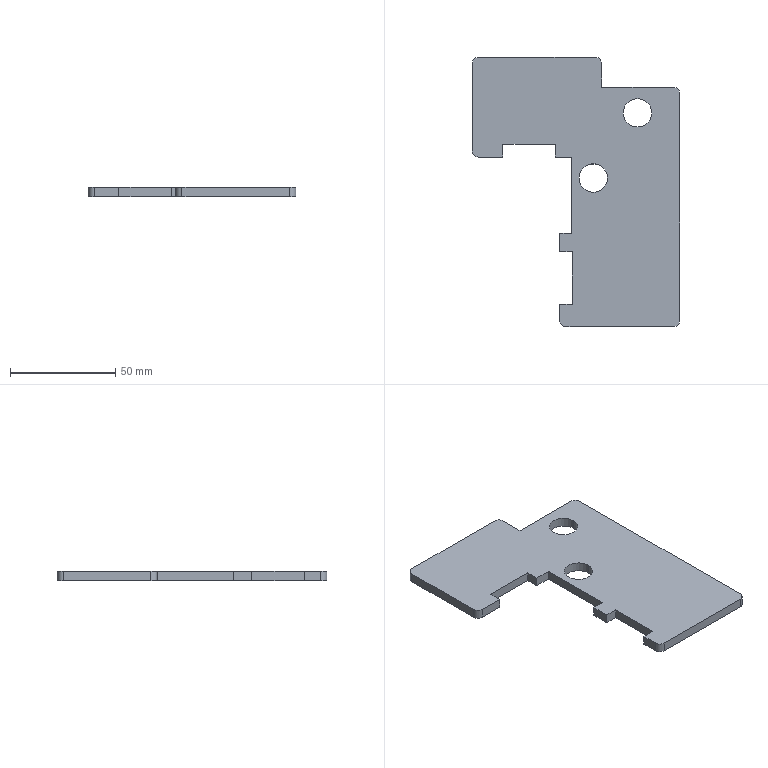Part | SolidWorks | features FlatPattern 1, SMBaseFlange 1, SheetMetal 1 | 1 solid | 30 faces | box 98.706 x 128.023 x 4.5 mm | volume 35781 mm3 | plane 20 | cylinder 10 | commonest cylinder face diameters 6 x6 13.5 x4
STEP:
#1=CARTESIAN_POINT('',(17799.004,-96072.131,-4.5));
#2=VERTEX_POINT('',#1);
#3=CARTESIAN_POINT('',(17812.504,-96072.131,-4.5));
#4=VERTEX_POINT('',#3);
#5=CARTESIAN_POINT('',(17805.754,-96072.131,-4.5));
#6=DIRECTION('',(0.,0.,1.));
#7=DIRECTION('',(1.,0.,0.));
#8=AXIS2_PLACEMENT_3D('',#5,#6,#7);
#9=CIRCLE('',#8,6.75);
#10=EDGE_CURVE('',#2,#4,#9,.T.);
#11=ORIENTED_EDGE('',*,*,#10,.F.);
#12=CARTESIAN_POINT('',(17799.004,-96072.131,0.));
#13=VERTEX_POINT('',#12);
#14=CARTESIAN_POINT('',(17799.004,-96072.131,-4.5));
#15=DIRECTION('',(0.,0.,1.));
#16=VECTOR('',#15,1000.);
#17=LINE('',#14,#16);
#18=EDGE_CURVE('',#2,#13,#17,.T.);
#19=ORIENTED_EDGE('',*,*,#18,.T.);
#20=CARTESIAN_POINT('',(17812.504,-96072.131,0.));
#21=VERTEX_POINT('',#20);
#22=CARTESIAN_POINT('',(17805.754,-96072.131,0.));
#23=DIRECTION('',(0.,0.,1.));
#24=DIRECTION('',(1.,0.,0.));
#25=AXIS2_PLACEMENT_3D('',#22,#23,#24);
#26=CIRCLE('',#25,6.75);
#27=EDGE_CURVE('',#13,#21,#26,.T.);
#28=ORIENTED_EDGE('',*,*,#27,.T.);
#29=CARTESIAN_POINT('',(17812.504,-96072.131,-4.5));
#30=DIRECTION('',(0.,0.,1.));
#31=VECTOR('',#30,1000.);
#32=LINE('',#29,#31);
#33=EDGE_CURVE('',#4,#21,#32,.T.);
#34=ORIENTED_EDGE('',*,*,#33,.F.);
#35=EDGE_LOOP('',(#11,#19,#28,#34));
#36=FACE_OUTER_BOUND('',#35,.T.);
#37=CARTESIAN_POINT('',(17805.754,-96072.131,-4.5));
#38=DIRECTION('',(0.,0.,1.));
#39=DIRECTION('',(1.,0.,0.));
#40=AXIS2_PLACEMENT_3D('',#37,#38,#39);
#41=CYLINDRICAL_SURFACE('',#40,6.75);
#42=ADVANCED_FACE('',(#36),#41,.F.);
#43=CARTESIAN_POINT('',(17778.004,-96103.131,-4.5));
#44=VERTEX_POINT('',#43);
#45=CARTESIAN_POINT('',(17791.504,-96103.131,-4.5));
#46=VERTEX_POINT('',#45);
#47=CARTESIAN_POINT('',(17784.754,-96103.131,-4.5));
#48=DIRECTION('',(0.,0.,1.));
#49=DIRECTION('',(1.,0.,0.));
#50=AXIS2_PLACEMENT_3D('',#47,#48,#49);
#51=CIRCLE('',#50,6.75);
#52=EDGE_CURVE('',#44,#46,#51,.T.);
#53=ORIENTED_EDGE('',*,*,#52,.F.);
#54=CARTESIAN_POINT('',(17778.004,-96103.131,0.));
#55=VERTEX_POINT('',#54);
#56=CARTESIAN_POINT('',(17778.004,-96103.131,-4.5));
#57=DIRECTION('',(0.,0.,1.));
#58=VECTOR('',#57,1000.);
#59=LINE('',#56,#58);
#60=EDGE_CURVE('',#44,#55,#59,.T.);
#61=ORIENTED_EDGE('',*,*,#60,.T.);
#62=CARTESIAN_POINT('',(17791.504,-96103.131,0.));
#63=VERTEX_POINT('',#62);
#64=CARTESIAN_POINT('',(17784.754,-96103.131,0.));
#65=DIRECTION('',(0.,0.,1.));
#66=DIRECTION('',(1.,0.,0.));
#67=AXIS2_PLACEMENT_3D('',#64,#65,#66);
#68=CIRCLE('',#67,6.75);
#69=EDGE_CURVE('',#55,#63,#68,.T.);
#70=ORIENTED_EDGE('',*,*,#69,.T.);
#71=CARTESIAN_POINT('',(17791.504,-96103.131,-4.5));
#72=DIRECTION('',(0.,0.,1.));
#73=VECTOR('',#72,1000.);
#74=LINE('',#71,#73);
#75=EDGE_CURVE('',#46,#63,#74,.T.);
#76=ORIENTED_EDGE('',*,*,#75,.F.);
#77=EDGE_LOOP('',(#53,#61,#70,#76));
#78=FACE_OUTER_BOUND('',#77,.T.);
#79=CARTESIAN_POINT('',(17784.754,-96103.131,-4.5));
#80=DIRECTION('',(0.,0.,1.));
#81=DIRECTION('',(1.,0.,0.));
#82=AXIS2_PLACEMENT_3D('',#79,#80,#81);
#83=CYLINDRICAL_SURFACE('',#82,6.75);
#84=ADVANCED_FACE('',(#78),#83,.F.);
#85=CARTESIAN_POINT('',(17730.162,-96045.724,0.));
#86=VERTEX_POINT('',#85);
#87=CARTESIAN_POINT('',(17727.162,-96048.724,0.));
#88=VERTEX_POINT('',#87);
#89=CARTESIAN_POINT('',(17730.162,-96048.724,0.));
#90=DIRECTION('',(0.,0.,1.));
#91=DIRECTION('',(-1.,0.,0.));
#92=AXIS2_PLACEMENT_3D('',#89,#90,#91);
#93=CIRCLE('',#92,3.);
#94=EDGE_CURVE('',#86,#88,#93,.T.);
#95=ORIENTED_EDGE('',*,*,#94,.F.);
#96=CARTESIAN_POINT('',(17730.162,-96045.724,-4.5));
#97=VERTEX_POINT('',#96);
#98=CARTESIAN_POINT('',(17730.162,-96045.724,-4.5));
#99=DIRECTION('',(0.,0.,1.));
#100=VECTOR('',#99,1000.);
#101=LINE('',#98,#100);
#102=EDGE_CURVE('',#97,#86,#101,.T.);
#103=ORIENTED_EDGE('',*,*,#102,.F.);
#104=CARTESIAN_POINT('',(17727.162,-96048.724,-4.5));
#105=VERTEX_POINT('',#104);
#106=CARTESIAN_POINT('',(17730.162,-96048.724,-4.5));
#107=DIRECTION('',(0.,0.,1.));
#108=DIRECTION('',(-1.,0.,0.));
#109=AXIS2_PLACEMENT_3D('',#106,#107,#108);
#110=CIRCLE('',#109,3.);
#111=EDGE_CURVE('',#97,#105,#110,.T.);
#112=ORIENTED_EDGE('',*,*,#111,.T.);
#113=CARTESIAN_POINT('',(17727.162,-96048.724,-4.5));
#114=DIRECTION('',(0.,0.,1.));
#115=VECTOR('',#114,1000.);
#116=LINE('',#113,#115);
#117=EDGE_CURVE('',#105,#88,#116,.T.);
#118=ORIENTED_EDGE('',*,*,#117,.T.);
#119=EDGE_LOOP('',(#95,#103,#112,#118));
#120=FACE_OUTER_BOUND('',#119,.T.);
#121=CARTESIAN_POINT('',(17730.162,-96048.724,-4.5));
#122=DIRECTION('',(0.,0.,1.));
#123=DIRECTION('',(1.,0.,0.));
#124=AXIS2_PLACEMENT_3D('',#121,#122,#123);
#125=CYLINDRICAL_SURFACE('',#124,3.);
#126=ADVANCED_FACE('',(#120),#125,.T.);
#127=CARTESIAN_POINT('',(17785.681,-96045.724,0.));
#128=VERTEX_POINT('',#127);
#129=CARTESIAN_POINT('',(17785.681,-96045.724,0.));
#130=DIRECTION('',(-1.,0.,0.));
#131=VECTOR('',#130,1000.);
#132=LINE('',#129,#131);
#133=EDGE_CURVE('',#128,#86,#132,.T.);
#134=ORIENTED_EDGE('',*,*,#133,.F.);
#135=CARTESIAN_POINT('',(17785.681,-96045.724,-4.5));
#136=VERTEX_POINT('',#135);
#137=CARTESIAN_POINT('',(17785.681,-96045.724,-4.5));
#138=DIRECTION('',(0.,0.,1.));
#139=VECTOR('',#138,1000.);
#140=LINE('',#137,#139);
#141=EDGE_CURVE('',#136,#128,#140,.T.);
#142=ORIENTED_EDGE('',*,*,#141,.F.);
#143=CARTESIAN_POINT('',(17785.681,-96045.724,-4.5));
#144=DIRECTION('',(-1.,0.,0.));
#145=VECTOR('',#144,1000.);
#146=LINE('',#143,#145);
#147=EDGE_CURVE('',#136,#97,#146,.T.);
#148=ORIENTED_EDGE('',*,*,#147,.T.);
#149=ORIENTED_EDGE('',*,*,#102,.T.);
#150=EDGE_LOOP('',(#134,#142,#148,#149));
#151=FACE_OUTER_BOUND('',#150,.T.);
#152=CARTESIAN_POINT('',(17785.681,-96045.724,-4.5));
#153=DIRECTION('',(0.,1.,0.));
#154=DIRECTION('',(0.,0.,1.));
#155=AXIS2_PLACEMENT_3D('',#152,#153,#154);
#156=PLANE('',#155);
#157=ADVANCED_FACE('',(#151),#156,.T.);
#158=CARTESIAN_POINT('',(17788.681,-96048.724,0.));
#159=VERTEX_POINT('',#158);
#160=CARTESIAN_POINT('',(17785.681,-96048.724,0.));
#161=DIRECTION('',(0.,0.,1.));
#162=DIRECTION('',(1.,0.,0.));
#163=AXIS2_PLACEMENT_3D('',#160,#161,#162);
#164=CIRCLE('',#163,3.);
#165=EDGE_CURVE('',#159,#128,#164,.T.);
#166=ORIENTED_EDGE('',*,*,#165,.F.);
#167=CARTESIAN_POINT('',(17788.681,-96048.724,-4.5));
#168=VERTEX_POINT('',#167);
#169=CARTESIAN_POINT('',(17788.681,-96048.724,-4.5));
#170=DIRECTION('',(0.,0.,1.));
#171=VECTOR('',#170,1000.);
#172=LINE('',#169,#171);
#173=EDGE_CURVE('',#168,#159,#172,.T.);
#174=ORIENTED_EDGE('',*,*,#173,.F.);
#175=CARTESIAN_POINT('',(17785.681,-96048.724,-4.5));
#176=DIRECTION('',(0.,0.,1.));
#177=DIRECTION('',(1.,0.,0.));
#178=AXIS2_PLACEMENT_3D('',#175,#176,#177);
#179=CIRCLE('',#178,3.);
#180=EDGE_CURVE('',#168,#136,#179,.T.);
#181=ORIENTED_EDGE('',*,*,#180,.T.);
#182=ORIENTED_EDGE('',*,*,#141,.T.);
#183=EDGE_LOOP('',(#166,#174,#181,#182));
#184=FACE_OUTER_BOUND('',#183,.T.);
#185=CARTESIAN_POINT('',(17785.681,-96048.724,-4.5));
#186=DIRECTION('',(0.,0.,1.));
#187=DIRECTION('',(1.,0.,0.));
#188=AXIS2_PLACEMENT_3D('',#185,#186,#187);
#189=CYLINDRICAL_SURFACE('',#188,3.);
#190=ADVANCED_FACE('',(#184),#189,.T.);
#191=CARTESIAN_POINT('',(17788.681,-96059.935,0.));
#192=VERTEX_POINT('',#191);
#193=CARTESIAN_POINT('',(17788.681,-96059.935,0.));
#194=DIRECTION('',(0.,1.,0.));
#195=VECTOR('',#194,1000.);
#196=LINE('',#193,#195);
#197=EDGE_CURVE('',#192,#159,#196,.T.);
#198=ORIENTED_EDGE('',*,*,#197,.F.);
#199=CARTESIAN_POINT('',(17788.681,-96059.935,-4.5));
#200=VERTEX_POINT('',#199);
#201=CARTESIAN_POINT('',(17788.681,-96059.935,-4.5));
#202=DIRECTION('',(0.,0.,1.));
#203=VECTOR('',#202,1000.);
#204=LINE('',#201,#203);
#205=EDGE_CURVE('',#200,#192,#204,.T.);
#206=ORIENTED_EDGE('',*,*,#205,.F.);
#207=CARTESIAN_POINT('',(17788.681,-96059.935,-4.5));
#208=DIRECTION('',(0.,1.,0.));
#209=VECTOR('',#208,1000.);
#210=LINE('',#207,#209);
#211=EDGE_CURVE('',#200,#168,#210,.T.);
#212=ORIENTED_EDGE('',*,*,#211,.T.);
#213=ORIENTED_EDGE('',*,*,#173,.T.);
#214=EDGE_LOOP('',(#198,#206,#212,#213));
#215=FACE_OUTER_BOUND('',#214,.T.);
#216=CARTESIAN_POINT('',(17788.681,-96059.935,-4.5));
#217=DIRECTION('',(1.,0.,0.));
#218=DIRECTION('',(0.,0.,-1.));
#219=AXIS2_PLACEMENT_3D('',#216,#217,#218);
#220=PLANE('',#219);
#221=ADVANCED_FACE('',(#215),#220,.T.);
#222=CARTESIAN_POINT('',(17822.868,-96059.935,0.));
#223=VERTEX_POINT('',#222);
#224=CARTESIAN_POINT('',(17822.868,-96059.935,0.));
#225=DIRECTION('',(-1.,0.,0.));
#226=VECTOR('',#225,1000.);
#227=LINE('',#224,#226);
#228=EDGE_CURVE('',#223,#192,#227,.T.);
#229=ORIENTED_EDGE('',*,*,#228,.F.);
#230=CARTESIAN_POINT('',(17822.868,-96059.935,-4.5));
#231=VERTEX_POINT('',#230);
#232=CARTESIAN_POINT('',(17822.868,-96059.935,-4.5));
#233=DIRECTION('',(0.,0.,1.));
#234=VECTOR('',#233,1000.);
#235=LINE('',#232,#234);
#236=EDGE_CURVE('',#231,#223,#235,.T.);
#237=ORIENTED_EDGE('',*,*,#236,.F.);
#238=CARTESIAN_POINT('',(17822.868,-96059.935,-4.5));
#239=DIRECTION('',(-1.,0.,0.));
#240=VECTOR('',#239,1000.);
#241=LINE('',#238,#240);
#242=EDGE_CURVE('',#231,#200,#241,.T.);
#243=ORIENTED_EDGE('',*,*,#242,.T.);
#244=ORIENTED_EDGE('',*,*,#205,.T.);
#245=EDGE_LOOP('',(#229,#237,#243,#244));
#246=FACE_OUTER_BOUND('',#245,.T.);
#247=CARTESIAN_POINT('',(17822.868,-96059.935,-4.5));
#248=DIRECTION('',(0.,1.,0.));
#249=DIRECTION('',(0.,0.,1.));
#250=AXIS2_PLACEMENT_3D('',#247,#248,#249);
#251=PLANE('',#250);
#252=ADVANCED_FACE('',(#246),#251,.T.);
#253=CARTESIAN_POINT('',(17825.868,-96062.935,0.));
#254=VERTEX_POINT('',#253);
#255=CARTESIAN_POINT('',(17822.868,-96062.935,0.));
#256=DIRECTION('',(0.,0.,1.));
#257=DIRECTION('',(1.,0.,0.));
#258=AXIS2_PLACEMENT_3D('',#255,#256,#257);
#259=CIRCLE('',#258,3.);
#260=EDGE_CURVE('',#254,#223,#259,.T.);
#261=ORIENTED_EDGE('',*,*,#260,.F.);
#262=CARTESIAN_POINT('',(17825.868,-96062.935,-4.5));
#263=VERTEX_POINT('',#262);
#264=CARTESIAN_POINT('',(17825.868,-96062.935,-4.5));
#265=DIRECTION('',(0.,0.,1.));
#266=VECTOR('',#265,1000.);
#267=LINE('',#264,#266);
#268=EDGE_CURVE('',#263,#254,#267,.T.);
#269=ORIENTED_EDGE('',*,*,#268,.F.);
#270=CARTESIAN_POINT('',(17822.868,-96062.935,-4.5));
#271=DIRECTION('',(0.,0.,1.));
#272=DIRECTION('',(1.,0.,0.));
#273=AXIS2_PLACEMENT_3D('',#270,#271,#272);
#274=CIRCLE('',#273,3.);
#275=EDGE_CURVE('',#263,#231,#274,.T.);
#276=ORIENTED_EDGE('',*,*,#275,.T.);
#277=ORIENTED_EDGE('',*,*,#236,.T.);
#278=EDGE_LOOP('',(#261,#269,#276,#277));
#279=FACE_OUTER_BOUND('',#278,.T.);
#280=CARTESIAN_POINT('',(17822.868,-96062.935,-4.5));
#281=DIRECTION('',(0.,0.,1.));
#282=DIRECTION('',(1.,0.,0.));
#283=AXIS2_PLACEMENT_3D('',#280,#281,#282);
#284=CYLINDRICAL_SURFACE('',#283,3.);
#285=ADVANCED_FACE('',(#279),#284,.T.);
#286=CARTESIAN_POINT('',(17825.868,-96170.747,0.));
#287=VERTEX_POINT('',#286);
#288=CARTESIAN_POINT('',(17825.868,-96062.935,0.));
#289=DIRECTION('',(0.,1.,0.));
#290=VECTOR('',#289,1000.);
#291=LINE('',#288,#290);
#292=EDGE_CURVE('',#287,#254,#291,.T.);
#293=ORIENTED_EDGE('',*,*,#292,.F.);
#294=CARTESIAN_POINT('',(17825.868,-96170.747,-4.5));
#295=VERTEX_POINT('',#294);
#296=CARTESIAN_POINT('',(17825.868,-96170.747,-4.5));
#297=DIRECTION('',(0.,0.,1.));
#298=VECTOR('',#297,1000.);
#299=LINE('',#296,#298);
#300=EDGE_CURVE('',#295,#287,#299,.T.);
#301=ORIENTED_EDGE('',*,*,#300,.F.);
#302=CARTESIAN_POINT('',(17825.868,-96062.935,-4.5));
#303=DIRECTION('',(0.,1.,0.));
#304=VECTOR('',#303,1000.);
#305=LINE('',#302,#304);
#306=EDGE_CURVE('',#295,#263,#305,.T.);
#307=ORIENTED_EDGE('',*,*,#306,.T.);
#308=ORIENTED_EDGE('',*,*,#268,.T.);
#309=EDGE_LOOP('',(#293,#301,#307,#308));
#310=FACE_OUTER_BOUND('',#309,.T.);
#311=CARTESIAN_POINT('',(17825.868,-96062.935,-4.5));
#312=DIRECTION('',(1.,0.,0.));
#313=DIRECTION('',(0.,1.,0.));
#314=AXIS2_PLACEMENT_3D('',#311,#312,#313);
#315=PLANE('',#314);
#316=ADVANCED_FACE('',(#310),#315,.T.);
#317=CARTESIAN_POINT('',(17822.868,-96173.747,0.));
#318=VERTEX_POINT('',#317);
#319=CARTESIAN_POINT('',(17822.868,-96170.747,0.));
#320=DIRECTION('',(0.,0.,1.));
#321=DIRECTION('',(1.,0.,0.));
#322=AXIS2_PLACEMENT_3D('',#319,#320,#321);
#323=CIRCLE('',#322,3.);
#324=EDGE_CURVE('',#318,#287,#323,.T.);
#325=ORIENTED_EDGE('',*,*,#324,.F.);
#326=CARTESIAN_POINT('',(17822.868,-96173.747,-4.5));
#327=VERTEX_POINT('',#326);
#328=CARTESIAN_POINT('',(17822.868,-96173.747,-4.5));
#329=DIRECTION('',(0.,0.,1.));
#330=VECTOR('',#329,1000.);
#331=LINE('',#328,#330);
#332=EDGE_CURVE('',#327,#318,#331,.T.);
#333=ORIENTED_EDGE('',*,*,#332,.F.);
#334=CARTESIAN_POINT('',(17822.868,-96170.747,-4.5));
#335=DIRECTION('',(0.,0.,1.));
#336=DIRECTION('',(1.,0.,0.));
#337=AXIS2_PLACEMENT_3D('',#334,#335,#336);
#338=CIRCLE('',#337,3.);
#339=EDGE_CURVE('',#327,#295,#338,.T.);
#340=ORIENTED_EDGE('',*,*,#339,.T.);
#341=ORIENTED_EDGE('',*,*,#300,.T.);
#342=EDGE_LOOP('',(#325,#333,#340,#341));
#343=FACE_OUTER_BOUND('',#342,.T.);
#344=CARTESIAN_POINT('',(17822.868,-96170.747,-4.5));
#345=DIRECTION('',(0.,0.,1.));
#346=DIRECTION('',(1.,0.,0.));
#347=AXIS2_PLACEMENT_3D('',#344,#345,#346);
#348=CYLINDRICAL_SURFACE('',#347,3.);
#349=ADVANCED_FACE('',(#343),#348,.T.);
#350=CARTESIAN_POINT('',(17771.754,-96173.747,0.));
#351=VERTEX_POINT('',#350);
#352=CARTESIAN_POINT('',(17822.868,-96173.747,0.));
#353=DIRECTION('',(1.,0.,0.));
#354=VECTOR('',#353,1000.);
#355=LINE('',#352,#354);
#356=EDGE_CURVE('',#351,#318,#355,.T.);
#357=ORIENTED_EDGE('',*,*,#356,.F.);
#358=CARTESIAN_POINT('',(17771.754,-96173.747,-4.5));
#359=VERTEX_POINT('',#358);
#360=CARTESIAN_POINT('',(17771.754,-96173.747,-4.5));
#361=DIRECTION('',(0.,0.,1.));
#362=VECTOR('',#361,1000.);
#363=LINE('',#360,#362);
#364=EDGE_CURVE('',#359,#351,#363,.T.);
#365=ORIENTED_EDGE('',*,*,#364,.F.);
#366=CARTESIAN_POINT('',(17822.868,-96173.747,-4.5));
#367=DIRECTION('',(1.,0.,0.));
#368=VECTOR('',#367,1000.);
#369=LINE('',#366,#368);
#370=EDGE_CURVE('',#359,#327,#369,.T.);
#371=ORIENTED_EDGE('',*,*,#370,.T.);
#372=ORIENTED_EDGE('',*,*,#332,.T.);
#373=EDGE_LOOP('',(#357,#365,#371,#372));
#374=FACE_OUTER_BOUND('',#373,.T.);
#375=CARTESIAN_POINT('',(17822.868,-96173.747,-4.5));
#376=DIRECTION('',(0.,-1.,0.));
#377=DIRECTION('',(1.,0.,0.));
#378=AXIS2_PLACEMENT_3D('',#375,#376,#377);
#379=PLANE('',#378);
#380=ADVANCED_FACE('',(#374),#379,.T.);
#381=CARTESIAN_POINT('',(17768.754,-96170.747,0.));
#382=VERTEX_POINT('',#381);
#383=CARTESIAN_POINT('',(17771.754,-96170.747,0.));
#384=DIRECTION('',(0.,0.,1.));
#385=DIRECTION('',(1.,0.,0.));
#386=AXIS2_PLACEMENT_3D('',#383,#384,#385);
#387=CIRCLE('',#386,3.);
#388=EDGE_CURVE('',#382,#351,#387,.T.);
#389=ORIENTED_EDGE('',*,*,#388,.F.);
#390=CARTESIAN_POINT('',(17768.754,-96170.747,-4.5));
#391=VERTEX_POINT('',#390);
#392=CARTESIAN_POINT('',(17768.754,-96170.747,-4.5));
#393=DIRECTION('',(0.,0.,1.));
#394=VECTOR('',#393,1000.);
#395=LINE('',#392,#394);
#396=EDGE_CURVE('',#391,#382,#395,.T.);
#397=ORIENTED_EDGE('',*,*,#396,.F.);
#398=CARTESIAN_POINT('',(17771.754,-96170.747,-4.5));
#399=DIRECTION('',(0.,0.,1.));
#400=DIRECTION('',(1.,0.,0.));
#401=AXIS2_PLACEMENT_3D('',#398,#399,#400);
#402=CIRCLE('',#401,3.);
#403=EDGE_CURVE('',#391,#359,#402,.T.);
#404=ORIENTED_EDGE('',*,*,#403,.T.);
#405=ORIENTED_EDGE('',*,*,#364,.T.);
#406=EDGE_LOOP('',(#389,#397,#404,#405));
#407=FACE_OUTER_BOUND('',#406,.T.);
#408=CARTESIAN_POINT('',(17771.754,-96170.747,-4.5));
#409=DIRECTION('',(0.,0.,1.));
#410=DIRECTION('',(1.,0.,0.));
#411=AXIS2_PLACEMENT_3D('',#408,#409,#410);
#412=CYLINDRICAL_SURFACE('',#411,3.);
#413=ADVANCED_FACE('',(#407),#412,.T.);
#414=CARTESIAN_POINT('',(17768.754,-96163.131,0.));
#415=VERTEX_POINT('',#414);
#416=CARTESIAN_POINT('',(17768.754,-96163.131,0.));
#417=DIRECTION('',(0.,-1.,0.));
#418=VECTOR('',#417,1000.);
#419=LINE('',#416,#418);
#420=EDGE_CURVE('',#415,#382,#419,.T.);
#421=ORIENTED_EDGE('',*,*,#420,.F.);
#422=CARTESIAN_POINT('',(17768.754,-96163.131,-4.5));
#423=VERTEX_POINT('',#422);
#424=CARTESIAN_POINT('',(17768.754,-96163.131,-4.5));
#425=DIRECTION('',(0.,0.,1.));
#426=VECTOR('',#425,1000.);
#427=LINE('',#424,#426);
#428=EDGE_CURVE('',#423,#415,#427,.T.);
#429=ORIENTED_EDGE('',*,*,#428,.F.);
#430=CARTESIAN_POINT('',(17768.754,-96163.131,-4.5));
#431=DIRECTION('',(0.,-1.,0.));
#432=VECTOR('',#431,1000.);
#433=LINE('',#430,#432);
#434=EDGE_CURVE('',#423,#391,#433,.T.);
#435=ORIENTED_EDGE('',*,*,#434,.T.);
#436=ORIENTED_EDGE('',*,*,#396,.T.);
#437=EDGE_LOOP('',(#421,#429,#435,#436));
#438=FACE_OUTER_BOUND('',#437,.T.);
#439=CARTESIAN_POINT('',(17768.754,-96163.131,-4.5));
#440=DIRECTION('',(-1.,0.,0.));
#441=DIRECTION('',(0.,0.,1.));
#442=AXIS2_PLACEMENT_3D('',#439,#440,#441);
#443=PLANE('',#442);
#444=ADVANCED_FACE('',(#438),#443,.T.);
#445=CARTESIAN_POINT('',(17774.754,-96163.131,0.));
#446=VERTEX_POINT('',#445);
#447=CARTESIAN_POINT('',(17774.754,-96163.131,0.));
#448=DIRECTION('',(-1.,0.,0.));
#449=VECTOR('',#448,1000.);
#450=LINE('',#447,#449);
#451=EDGE_CURVE('',#446,#415,#450,.T.);
#452=ORIENTED_EDGE('',*,*,#451,.F.);
#453=CARTESIAN_POINT('',(17774.754,-96163.131,-4.5));
#454=VERTEX_POINT('',#453);
#455=CARTESIAN_POINT('',(17774.754,-96163.131,-4.5));
#456=DIRECTION('',(0.,0.,1.));
#457=VECTOR('',#456,1000.);
#458=LINE('',#455,#457);
#459=EDGE_CURVE('',#454,#446,#458,.T.);
#460=ORIENTED_EDGE('',*,*,#459,.F.);
#461=CARTESIAN_POINT('',(17774.754,-96163.131,-4.5));
#462=DIRECTION('',(-1.,0.,0.));
#463=VECTOR('',#462,1000.);
#464=LINE('',#461,#463);
#465=EDGE_CURVE('',#454,#423,#464,.T.);
#466=ORIENTED_EDGE('',*,*,#465,.T.);
#467=ORIENTED_EDGE('',*,*,#428,.T.);
#468=EDGE_LOOP('',(#452,#460,#466,#467));
#469=FACE_OUTER_BOUND('',#468,.T.);
#470=CARTESIAN_POINT('',(17774.754,-96163.131,-4.5));
#471=DIRECTION('',(0.,1.,0.));
#472=DIRECTION('',(0.,0.,1.));
#473=AXIS2_PLACEMENT_3D('',#470,#471,#472);
#474=PLANE('',#473);
#475=ADVANCED_FACE('',(#469),#474,.T.);
#476=CARTESIAN_POINT('',(17774.754,-96138.131,0.));
#477=VERTEX_POINT('',#476);
#478=CARTESIAN_POINT('',(17774.754,-96138.131,0.));
#479=DIRECTION('',(0.,-1.,0.));
#480=VECTOR('',#479,1000.);
#481=LINE('',#478,#480);
#482=EDGE_CURVE('',#477,#446,#481,.T.);
#483=ORIENTED_EDGE('',*,*,#482,.F.);
#484=CARTESIAN_POINT('',(17774.754,-96138.131,-4.5));
#485=VERTEX_POINT('',#484);
#486=CARTESIAN_POINT('',(17774.754,-96138.131,-4.5));
#487=DIRECTION('',(0.,0.,1.));
#488=VECTOR('',#487,1000.);
#489=LINE('',#486,#488);
#490=EDGE_CURVE('',#485,#477,#489,.T.);
#491=ORIENTED_EDGE('',*,*,#490,.F.);
#492=CARTESIAN_POINT('',(17774.754,-96138.131,-4.5));
#493=DIRECTION('',(0.,-1.,0.));
#494=VECTOR('',#493,1000.);
#495=LINE('',#492,#494);
#496=EDGE_CURVE('',#485,#454,#495,.T.);
#497=ORIENTED_EDGE('',*,*,#496,.T.);
#498=ORIENTED_EDGE('',*,*,#459,.T.);
#499=EDGE_LOOP('',(#483,#491,#497,#498));
#500=FACE_OUTER_BOUND('',#499,.T.);
#501=CARTESIAN_POINT('',(17774.754,-96138.131,-4.5));
#502=DIRECTION('',(-1.,0.,0.));
#503=DIRECTION('',(0.,0.,1.));
#504=AXIS2_PLACEMENT_3D('',#501,#502,#503);
#505=PLANE('',#504);
#506=ADVANCED_FACE('',(#500),#505,.T.);
#507=CARTESIAN_POINT('',(17768.754,-96138.131,0.));
#508=VERTEX_POINT('',#507);
#509=CARTESIAN_POINT('',(17774.754,-96138.131,0.));
#510=DIRECTION('',(1.,0.,0.));
#511=VECTOR('',#510,1000.);
#512=LINE('',#509,#511);
#513=EDGE_CURVE('',#508,#477,#512,.T.);
#514=ORIENTED_EDGE('',*,*,#513,.F.);
#515=CARTESIAN_POINT('',(17768.754,-96138.131,-4.5));
#516=VERTEX_POINT('',#515);
#517=CARTESIAN_POINT('',(17768.754,-96138.131,-4.5));
#518=DIRECTION('',(0.,0.,1.));
#519=VECTOR('',#518,1000.);
#520=LINE('',#517,#519);
#521=EDGE_CURVE('',#516,#508,#520,.T.);
#522=ORIENTED_EDGE('',*,*,#521,.F.);
#523=CARTESIAN_POINT('',(17774.754,-96138.131,-4.5));
#524=DIRECTION('',(1.,0.,0.));
#525=VECTOR('',#524,1000.);
#526=LINE('',#523,#525);
#527=EDGE_CURVE('',#516,#485,#526,.T.);
#528=ORIENTED_EDGE('',*,*,#527,.T.);
#529=ORIENTED_EDGE('',*,*,#490,.T.);
#530=EDGE_LOOP('',(#514,#522,#528,#529));
#531=FACE_OUTER_BOUND('',#530,.T.);
#532=CARTESIAN_POINT('',(17774.754,-96138.131,-4.5));
#533=DIRECTION('',(0.,-1.,0.));
#534=DIRECTION('',(1.,0.,0.));
#535=AXIS2_PLACEMENT_3D('',#532,#533,#534);
#536=PLANE('',#535);
#537=ADVANCED_FACE('',(#531),#536,.T.);
#538=CARTESIAN_POINT('',(17768.754,-96129.43,0.));
#539=VERTEX_POINT('',#538);
#540=CARTESIAN_POINT('',(17768.754,-96129.43,0.));
#541=DIRECTION('',(0.,-1.,0.));
#542=VECTOR('',#541,1000.);
#543=LINE('',#540,#542);
#544=EDGE_CURVE('',#539,#508,#543,.T.);
#545=ORIENTED_EDGE('',*,*,#544,.F.);
#546=CARTESIAN_POINT('',(17768.754,-96129.43,-4.5));
#547=VERTEX_POINT('',#546);
#548=CARTESIAN_POINT('',(17768.754,-96129.43,-4.5));
#549=DIRECTION('',(0.,0.,1.));
#550=VECTOR('',#549,1000.);
#551=LINE('',#548,#550);
#552=EDGE_CURVE('',#547,#539,#551,.T.);
#553=ORIENTED_EDGE('',*,*,#552,.F.);
#554=CARTESIAN_POINT('',(17768.754,-96129.43,-4.5));
#555=DIRECTION('',(0.,-1.,0.));
#556=VECTOR('',#555,1000.);
#557=LINE('',#554,#556);
#558=EDGE_CURVE('',#547,#516,#557,.T.);
#559=ORIENTED_EDGE('',*,*,#558,.T.);
#560=ORIENTED_EDGE('',*,*,#521,.T.);
#561=EDGE_LOOP('',(#545,#553,#559,#560));
#562=FACE_OUTER_BOUND('',#561,.T.);
#563=CARTESIAN_POINT('',(17768.754,-96129.43,-4.5));
#564=DIRECTION('',(-1.,0.,0.));
#565=DIRECTION('',(0.,0.,1.));
#566=AXIS2_PLACEMENT_3D('',#563,#564,#565);
#567=PLANE('',#566);
#568=ADVANCED_FACE('',(#562),#567,.T.);
#569=CARTESIAN_POINT('',(17774.431,-96129.43,0.));
#570=VERTEX_POINT('',#569);
#571=CARTESIAN_POINT('',(17774.431,-96129.43,0.));
#572=DIRECTION('',(-1.,0.,0.));
#573=VECTOR('',#572,1000.);
#574=LINE('',#571,#573);
#575=EDGE_CURVE('',#570,#539,#574,.T.);
#576=ORIENTED_EDGE('',*,*,#575,.F.);
#577=CARTESIAN_POINT('',(17774.431,-96129.43,-4.5));
#578=VERTEX_POINT('',#577);
#579=CARTESIAN_POINT('',(17774.431,-96129.43,-4.5));
#580=DIRECTION('',(0.,0.,1.));
#581=VECTOR('',#580,1000.);
#582=LINE('',#579,#581);
#583=EDGE_CURVE('',#578,#570,#582,.T.);
#584=ORIENTED_EDGE('',*,*,#583,.F.);
#585=CARTESIAN_POINT('',(17774.431,-96129.43,-4.5));
#586=DIRECTION('',(-1.,0.,0.));
#587=VECTOR('',#586,1000.);
#588=LINE('',#585,#587);
#589=EDGE_CURVE('',#578,#547,#588,.T.);
#590=ORIENTED_EDGE('',*,*,#589,.T.);
#591=ORIENTED_EDGE('',*,*,#552,.T.);
#592=EDGE_LOOP('',(#576,#584,#590,#591));
#593=FACE_OUTER_BOUND('',#592,.T.);
#594=CARTESIAN_POINT('',(17774.431,-96129.43,-4.5));
#595=DIRECTION('',(0.,1.,0.));
#596=DIRECTION('',(-1.,0.,0.));
#597=AXIS2_PLACEMENT_3D('',#594,#595,#596);
#598=PLANE('',#597);
#599=ADVANCED_FACE('',(#593),#598,.T.);
#600=CARTESIAN_POINT('',(17774.431,-96093.131,0.));
#601=VERTEX_POINT('',#600);
#602=CARTESIAN_POINT('',(17774.431,-96093.131,0.));
#603=DIRECTION('',(0.,-1.,0.));
#604=VECTOR('',#603,1000.);
#605=LINE('',#602,#604);
#606=EDGE_CURVE('',#601,#570,#605,.T.);
#607=ORIENTED_EDGE('',*,*,#606,.F.);
#608=CARTESIAN_POINT('',(17774.431,-96093.131,-4.5));
#609=VERTEX_POINT('',#608);
#610=CARTESIAN_POINT('',(17774.431,-96093.131,-4.5));
#611=DIRECTION('',(0.,0.,1.));
#612=VECTOR('',#611,1000.);
#613=LINE('',#610,#612);
#614=EDGE_CURVE('',#609,#601,#613,.T.);
#615=ORIENTED_EDGE('',*,*,#614,.F.);
#616=CARTESIAN_POINT('',(17774.431,-96093.131,-4.5));
#617=DIRECTION('',(0.,-1.,0.));
#618=VECTOR('',#617,1000.);
#619=LINE('',#616,#618);
#620=EDGE_CURVE('',#609,#578,#619,.T.);
#621=ORIENTED_EDGE('',*,*,#620,.T.);
#622=ORIENTED_EDGE('',*,*,#583,.T.);
#623=EDGE_LOOP('',(#607,#615,#621,#622));
#624=FACE_OUTER_BOUND('',#623,.T.);
#625=CARTESIAN_POINT('',(17774.431,-96093.131,-4.5));
#626=DIRECTION('',(-1.,0.,0.));
#627=DIRECTION('',(0.,0.,1.));
#628=AXIS2_PLACEMENT_3D('',#625,#626,#627);
#629=PLANE('',#628);
#630=ADVANCED_FACE('',(#624),#629,.T.);
#631=CARTESIAN_POINT('',(17766.754,-96093.131,0.));
#632=VERTEX_POINT('',#631);
#633=CARTESIAN_POINT('',(17766.754,-96093.131,0.));
#634=DIRECTION('',(1.,0.,0.));
#635=VECTOR('',#634,1000.);
#636=LINE('',#633,#635);
#637=EDGE_CURVE('',#632,#601,#636,.T.);
#638=ORIENTED_EDGE('',*,*,#637,.F.);
#639=CARTESIAN_POINT('',(17766.754,-96093.131,-4.5));
#640=VERTEX_POINT('',#639);
#641=CARTESIAN_POINT('',(17766.754,-96093.131,-4.5));
#642=DIRECTION('',(0.,0.,1.));
#643=VECTOR('',#642,1000.);
#644=LINE('',#641,#643);
#645=EDGE_CURVE('',#640,#632,#644,.T.);
#646=ORIENTED_EDGE('',*,*,#645,.F.);
#647=CARTESIAN_POINT('',(17766.754,-96093.131,-4.5));
#648=DIRECTION('',(1.,0.,0.));
#649=VECTOR('',#648,1000.);
#650=LINE('',#647,#649);
#651=EDGE_CURVE('',#640,#609,#650,.T.);
#652=ORIENTED_EDGE('',*,*,#651,.T.);
#653=ORIENTED_EDGE('',*,*,#614,.T.);
#654=EDGE_LOOP('',(#638,#646,#652,#653));
#655=FACE_OUTER_BOUND('',#654,.T.);
#656=CARTESIAN_POINT('',(17766.754,-96093.131,-4.5));
#657=DIRECTION('',(0.,-1.,0.));
#658=DIRECTION('',(1.,0.,0.));
#659=AXIS2_PLACEMENT_3D('',#656,#657,#658);
#660=PLANE('',#659);
#661=ADVANCED_FACE('',(#655),#660,.T.);
#662=CARTESIAN_POINT('',(17766.754,-96087.131,0.));
#663=VERTEX_POINT('',#662);
#664=CARTESIAN_POINT('',(17766.754,-96093.131,0.));
#665=DIRECTION('',(0.,-1.,0.));
#666=VECTOR('',#665,1000.);
#667=LINE('',#664,#666);
#668=EDGE_CURVE('',#663,#632,#667,.T.);
#669=ORIENTED_EDGE('',*,*,#668,.F.);
#670=CARTESIAN_POINT('',(17766.754,-96087.131,-4.5));
#671=VERTEX_POINT('',#670);
#672=CARTESIAN_POINT('',(17766.754,-96087.131,-4.5));
#673=DIRECTION('',(0.,0.,1.));
#674=VECTOR('',#673,1000.);
#675=LINE('',#672,#674);
#676=EDGE_CURVE('',#671,#663,#675,.T.);
#677=ORIENTED_EDGE('',*,*,#676,.F.);
#678=CARTESIAN_POINT('',(17766.754,-96093.131,-4.5));
#679=DIRECTION('',(0.,-1.,0.));
#680=VECTOR('',#679,1000.);
#681=LINE('',#678,#680);
#682=EDGE_CURVE('',#671,#640,#681,.T.);
#683=ORIENTED_EDGE('',*,*,#682,.T.);
#684=ORIENTED_EDGE('',*,*,#645,.T.);
#685=EDGE_LOOP('',(#669,#677,#683,#684));
#686=FACE_OUTER_BOUND('',#685,.T.);
#687=CARTESIAN_POINT('',(17766.754,-96093.131,-4.5));
#688=DIRECTION('',(-1.,0.,0.));
#689=DIRECTION('',(0.,0.,1.));
#690=AXIS2_PLACEMENT_3D('',#687,#688,#689);
#691=PLANE('',#690);
#692=ADVANCED_FACE('',(#686),#691,.T.);
#693=CARTESIAN_POINT('',(17741.754,-96087.131,0.));
#694=VERTEX_POINT('',#693);
#695=CARTESIAN_POINT('',(17741.754,-96087.131,0.));
#696=DIRECTION('',(1.,0.,0.));
#697=VECTOR('',#696,1000.);
#698=LINE('',#695,#697);
#699=EDGE_CURVE('',#694,#663,#698,.T.);
#700=ORIENTED_EDGE('',*,*,#699,.F.);
#701=CARTESIAN_POINT('',(17741.754,-96087.131,-4.5));
#702=VERTEX_POINT('',#701);
#703=CARTESIAN_POINT('',(17741.754,-96087.131,-4.5));
#704=DIRECTION('',(0.,0.,1.));
#705=VECTOR('',#704,1000.);
#706=LINE('',#703,#705);
#707=EDGE_CURVE('',#702,#694,#706,.T.);
#708=ORIENTED_EDGE('',*,*,#707,.F.);
#709=CARTESIAN_POINT('',(17741.754,-96087.131,-4.5));
#710=DIRECTION('',(1.,0.,0.));
#711=VECTOR('',#710,1000.);
#712=LINE('',#709,#711);
#713=EDGE_CURVE('',#702,#671,#712,.T.);
#714=ORIENTED_EDGE('',*,*,#713,.T.);
#715=ORIENTED_EDGE('',*,*,#676,.T.);
#716=EDGE_LOOP('',(#700,#708,#714,#715));
#717=FACE_OUTER_BOUND('',#716,.T.);
#718=CARTESIAN_POINT('',(17741.754,-96087.131,-4.5));
#719=DIRECTION('',(0.,-1.,0.));
#720=DIRECTION('',(1.,0.,0.));
#721=AXIS2_PLACEMENT_3D('',#718,#719,#720);
#722=PLANE('',#721);
#723=ADVANCED_FACE('',(#717),#722,.T.);
#724=CARTESIAN_POINT('',(17741.754,-96093.131,0.));
#725=VERTEX_POINT('',#724);
#726=CARTESIAN_POINT('',(17741.754,-96093.131,0.));
#727=DIRECTION('',(0.,1.,0.));
#728=VECTOR('',#727,1000.);
#729=LINE('',#726,#728);
#730=EDGE_CURVE('',#725,#694,#729,.T.);
#731=ORIENTED_EDGE('',*,*,#730,.F.);
#732=CARTESIAN_POINT('',(17741.754,-96093.131,-4.5));
#733=VERTEX_POINT('',#732);
#734=CARTESIAN_POINT('',(17741.754,-96093.131,-4.5));
#735=DIRECTION('',(0.,0.,1.));
#736=VECTOR('',#735,1000.);
#737=LINE('',#734,#736);
#738=EDGE_CURVE('',#733,#725,#737,.T.);
#739=ORIENTED_EDGE('',*,*,#738,.F.);
#740=CARTESIAN_POINT('',(17741.754,-96093.131,-4.5));
#741=DIRECTION('',(0.,1.,0.));
#742=VECTOR('',#741,1000.);
#743=LINE('',#740,#742);
#744=EDGE_CURVE('',#733,#702,#743,.T.);
#745=ORIENTED_EDGE('',*,*,#744,.T.);
#746=ORIENTED_EDGE('',*,*,#707,.T.);
#747=EDGE_LOOP('',(#731,#739,#745,#746));
#748=FACE_OUTER_BOUND('',#747,.T.);
#749=CARTESIAN_POINT('',(17741.754,-96093.131,-4.5));
#750=DIRECTION('',(1.,0.,0.));
#751=DIRECTION('',(0.,0.,-1.));
#752=AXIS2_PLACEMENT_3D('',#749,#750,#751);
#753=PLANE('',#752);
#754=ADVANCED_FACE('',(#748),#753,.T.);
#755=CARTESIAN_POINT('',(17730.162,-96093.131,0.));
#756=VERTEX_POINT('',#755);
#757=CARTESIAN_POINT('',(17730.162,-96093.131,0.));
#758=DIRECTION('',(1.,0.,0.));
#759=VECTOR('',#758,1000.);
#760=LINE('',#757,#759);
#761=EDGE_CURVE('',#756,#725,#760,.T.);
#762=ORIENTED_EDGE('',*,*,#761,.F.);
#763=CARTESIAN_POINT('',(17730.162,-96093.131,-4.5));
#764=VERTEX_POINT('',#763);
#765=CARTESIAN_POINT('',(17730.162,-96093.131,-4.5));
#766=DIRECTION('',(0.,0.,1.));
#767=VECTOR('',#766,1000.);
#768=LINE('',#765,#767);
#769=EDGE_CURVE('',#764,#756,#768,.T.);
#770=ORIENTED_EDGE('',*,*,#769,.F.);
#771=CARTESIAN_POINT('',(17730.162,-96093.131,-4.5));
#772=DIRECTION('',(1.,0.,0.));
#773=VECTOR('',#772,1000.);
#774=LINE('',#771,#773);
#775=EDGE_CURVE('',#764,#733,#774,.T.);
#776=ORIENTED_EDGE('',*,*,#775,.T.);
#777=ORIENTED_EDGE('',*,*,#738,.T.);
#778=EDGE_LOOP('',(#762,#770,#776,#777));
#779=FACE_OUTER_BOUND('',#778,.T.);
#780=CARTESIAN_POINT('',(17730.162,-96093.131,-4.5));
#781=DIRECTION('',(0.,-1.,0.));
#782=DIRECTION('',(1.,0.,0.));
#783=AXIS2_PLACEMENT_3D('',#780,#781,#782);
#784=PLANE('',#783);
#785=ADVANCED_FACE('',(#779),#784,.T.);
#786=CARTESIAN_POINT('',(17727.162,-96090.131,0.));
#787=VERTEX_POINT('',#786);
#788=CARTESIAN_POINT('',(17730.162,-96090.131,0.));
#789=DIRECTION('',(0.,0.,1.));
#790=DIRECTION('',(1.,0.,0.));
#791=AXIS2_PLACEMENT_3D('',#788,#789,#790);
#792=CIRCLE('',#791,3.);
#793=EDGE_CURVE('',#787,#756,#792,.T.);
#794=ORIENTED_EDGE('',*,*,#793,.F.);
#795=CARTESIAN_POINT('',(17727.162,-96090.131,-4.5));
#796=VERTEX_POINT('',#795);
#797=CARTESIAN_POINT('',(17727.162,-96090.131,-4.5));
#798=DIRECTION('',(0.,0.,1.));
#799=VECTOR('',#798,1000.);
#800=LINE('',#797,#799);
#801=EDGE_CURVE('',#796,#787,#800,.T.);
#802=ORIENTED_EDGE('',*,*,#801,.F.);
#803=CARTESIAN_POINT('',(17730.162,-96090.131,-4.5));
#804=DIRECTION('',(0.,0.,1.));
#805=DIRECTION('',(1.,0.,0.));
#806=AXIS2_PLACEMENT_3D('',#803,#804,#805);
#807=CIRCLE('',#806,3.);
#808=EDGE_CURVE('',#796,#764,#807,.T.);
#809=ORIENTED_EDGE('',*,*,#808,.T.);
#810=ORIENTED_EDGE('',*,*,#769,.T.);
#811=EDGE_LOOP('',(#794,#802,#809,#810));
#812=FACE_OUTER_BOUND('',#811,.T.);
#813=CARTESIAN_POINT('',(17730.162,-96090.131,-4.5));
#814=DIRECTION('',(0.,0.,1.));
#815=DIRECTION('',(1.,0.,0.));
#816=AXIS2_PLACEMENT_3D('',#813,#814,#815);
#817=CYLINDRICAL_SURFACE('',#816,3.);
#818=ADVANCED_FACE('',(#812),#817,.T.);
#819=CARTESIAN_POINT('',(17727.162,-96090.131,0.));
#820=DIRECTION('',(0.,-1.,0.));
#821=VECTOR('',#820,1000.);
#822=LINE('',#819,#821);
#823=EDGE_CURVE('',#88,#787,#822,.T.);
#824=ORIENTED_EDGE('',*,*,#823,.F.);
#825=ORIENTED_EDGE('',*,*,#117,.F.);
#826=CARTESIAN_POINT('',(17727.162,-96090.131,-4.5));
#827=DIRECTION('',(0.,-1.,0.));
#828=VECTOR('',#827,1000.);
#829=LINE('',#826,#828);
#830=EDGE_CURVE('',#105,#796,#829,.T.);
#831=ORIENTED_EDGE('',*,*,#830,.T.);
#832=ORIENTED_EDGE('',*,*,#801,.T.);
#833=EDGE_LOOP('',(#824,#825,#831,#832));
#834=FACE_OUTER_BOUND('',#833,.T.);
#835=CARTESIAN_POINT('',(17727.162,-96090.131,-4.5));
#836=DIRECTION('',(-1.,0.,0.));
#837=DIRECTION('',(0.,0.,1.));
#838=AXIS2_PLACEMENT_3D('',#835,#836,#837);
#839=PLANE('',#838);
#840=ADVANCED_FACE('',(#834),#839,.T.);
#841=CARTESIAN_POINT('',(17805.754,-96072.131,-4.5));
#842=DIRECTION('',(0.,0.,1.));
#843=DIRECTION('',(1.,0.,0.));
#844=AXIS2_PLACEMENT_3D('',#841,#842,#843);
#845=CIRCLE('',#844,6.75);
#846=EDGE_CURVE('',#4,#2,#845,.T.);
#847=ORIENTED_EDGE('',*,*,#846,.T.);
#848=ORIENTED_EDGE('',*,*,#10,.T.);
#849=EDGE_LOOP('',(#847,#848));
#850=FACE_BOUND('',#849,.T.);
#851=CARTESIAN_POINT('',(17784.754,-96103.131,-4.5));
#852=DIRECTION('',(0.,0.,1.));
#853=DIRECTION('',(1.,0.,0.));
#854=AXIS2_PLACEMENT_3D('',#851,#852,#853);
#855=CIRCLE('',#854,6.75);
#856=EDGE_CURVE('',#46,#44,#855,.T.);
#857=ORIENTED_EDGE('',*,*,#856,.T.);
#858=ORIENTED_EDGE('',*,*,#52,.T.);
#859=EDGE_LOOP('',(#857,#858));
#860=FACE_BOUND('',#859,.T.);
#861=ORIENTED_EDGE('',*,*,#111,.F.);
#862=ORIENTED_EDGE('',*,*,#147,.F.);
#863=ORIENTED_EDGE('',*,*,#180,.F.);
#864=ORIENTED_EDGE('',*,*,#211,.F.);
#865=ORIENTED_EDGE('',*,*,#242,.F.);
#866=ORIENTED_EDGE('',*,*,#275,.F.);
#867=ORIENTED_EDGE('',*,*,#306,.F.);
#868=ORIENTED_EDGE('',*,*,#339,.F.);
#869=ORIENTED_EDGE('',*,*,#370,.F.);
#870=ORIENTED_EDGE('',*,*,#403,.F.);
#871=ORIENTED_EDGE('',*,*,#434,.F.);
#872=ORIENTED_EDGE('',*,*,#465,.F.);
#873=ORIENTED_EDGE('',*,*,#496,.F.);
#874=ORIENTED_EDGE('',*,*,#527,.F.);
#875=ORIENTED_EDGE('',*,*,#558,.F.);
#876=ORIENTED_EDGE('',*,*,#589,.F.);
#877=ORIENTED_EDGE('',*,*,#620,.F.);
#878=ORIENTED_EDGE('',*,*,#651,.F.);
#879=ORIENTED_EDGE('',*,*,#682,.F.);
#880=ORIENTED_EDGE('',*,*,#713,.F.);
#881=ORIENTED_EDGE('',*,*,#744,.F.);
#882=ORIENTED_EDGE('',*,*,#775,.F.);
#883=ORIENTED_EDGE('',*,*,#808,.F.);
#884=ORIENTED_EDGE('',*,*,#830,.F.);
#885=EDGE_LOOP('',(#861,#862,#863,#864,#865,#866,#867,#868,#869,#870,#871,#872,#873,#874,#875,#876,#877,#878,#879,#880,#881,#882,#883,#884));
#886=FACE_OUTER_BOUND('',#885,.T.);
#887=CARTESIAN_POINT('',(17730.162,-96048.724,-4.5));
#888=DIRECTION('',(0.,0.,-1.));
#889=DIRECTION('',(-1.,0.,0.));
#890=AXIS2_PLACEMENT_3D('',#887,#888,#889);
#891=PLANE('',#890);
#892=ADVANCED_FACE('',(#850,#860,#886),#891,.T.);
#893=CARTESIAN_POINT('',(17805.754,-96072.131,0.));
#894=DIRECTION('',(0.,0.,1.));
#895=DIRECTION('',(1.,0.,0.));
#896=AXIS2_PLACEMENT_3D('',#893,#894,#895);
#897=CIRCLE('',#896,6.75);
#898=EDGE_CURVE('',#21,#13,#897,.T.);
#899=ORIENTED_EDGE('',*,*,#898,.F.);
#900=ORIENTED_EDGE('',*,*,#27,.F.);
#901=EDGE_LOOP('',(#899,#900));
#902=FACE_BOUND('',#901,.T.);
#903=CARTESIAN_POINT('',(17784.754,-96103.131,0.));
#904=DIRECTION('',(0.,0.,1.));
#905=DIRECTION('',(1.,0.,0.));
#906=AXIS2_PLACEMENT_3D('',#903,#904,#905);
#907=CIRCLE('',#906,6.75);
#908=EDGE_CURVE('',#63,#55,#907,.T.);
#909=ORIENTED_EDGE('',*,*,#908,.F.);
#910=ORIENTED_EDGE('',*,*,#69,.F.);
#911=EDGE_LOOP('',(#909,#910));
#912=FACE_BOUND('',#911,.T.);
#913=ORIENTED_EDGE('',*,*,#94,.T.);
#914=ORIENTED_EDGE('',*,*,#823,.T.);
#915=ORIENTED_EDGE('',*,*,#793,.T.);
#916=ORIENTED_EDGE('',*,*,#761,.T.);
#917=ORIENTED_EDGE('',*,*,#730,.T.);
#918=ORIENTED_EDGE('',*,*,#699,.T.);
#919=ORIENTED_EDGE('',*,*,#668,.T.);
#920=ORIENTED_EDGE('',*,*,#637,.T.);
#921=ORIENTED_EDGE('',*,*,#606,.T.);
#922=ORIENTED_EDGE('',*,*,#575,.T.);
#923=ORIENTED_EDGE('',*,*,#544,.T.);
#924=ORIENTED_EDGE('',*,*,#513,.T.);
#925=ORIENTED_EDGE('',*,*,#482,.T.);
#926=ORIENTED_EDGE('',*,*,#451,.T.);
#927=ORIENTED_EDGE('',*,*,#420,.T.);
#928=ORIENTED_EDGE('',*,*,#388,.T.);
#929=ORIENTED_EDGE('',*,*,#356,.T.);
#930=ORIENTED_EDGE('',*,*,#324,.T.);
#931=ORIENTED_EDGE('',*,*,#292,.T.);
#932=ORIENTED_EDGE('',*,*,#260,.T.);
#933=ORIENTED_EDGE('',*,*,#228,.T.);
#934=ORIENTED_EDGE('',*,*,#197,.T.);
#935=ORIENTED_EDGE('',*,*,#165,.T.);
#936=ORIENTED_EDGE('',*,*,#133,.T.);
#937=EDGE_LOOP('',(#913,#914,#915,#916,#917,#918,#919,#920,#921,#922,#923,#924,#925,#926,#927,#928,#929,#930,#931,#932,#933,#934,#935,#936));
#938=FACE_OUTER_BOUND('',#937,.T.);
#939=CARTESIAN_POINT('',(17730.162,-96048.724,0.));
#940=DIRECTION('',(0.,0.,-1.));
#941=DIRECTION('',(-1.,0.,0.));
#942=AXIS2_PLACEMENT_3D('',#939,#940,#941);
#943=PLANE('',#942);
#944=ADVANCED_FACE('',(#902,#912,#938),#943,.F.);
#945=ORIENTED_EDGE('',*,*,#60,.F.);
#946=ORIENTED_EDGE('',*,*,#856,.F.);
#947=ORIENTED_EDGE('',*,*,#75,.T.);
#948=ORIENTED_EDGE('',*,*,#908,.T.);
#949=EDGE_LOOP('',(#945,#946,#947,#948));
#950=FACE_OUTER_BOUND('',#949,.T.);
#951=CARTESIAN_POINT('',(17784.754,-96103.131,-4.5));
#952=DIRECTION('',(0.,0.,1.));
#953=DIRECTION('',(1.,0.,0.));
#954=AXIS2_PLACEMENT_3D('',#951,#952,#953);
#955=CYLINDRICAL_SURFACE('',#954,6.75);
#956=ADVANCED_FACE('',(#950),#955,.F.);
#957=ORIENTED_EDGE('',*,*,#18,.F.);
#958=ORIENTED_EDGE('',*,*,#846,.F.);
#959=ORIENTED_EDGE('',*,*,#33,.T.);
#960=ORIENTED_EDGE('',*,*,#898,.T.);
#961=EDGE_LOOP('',(#957,#958,#959,#960));
#962=FACE_OUTER_BOUND('',#961,.T.);
#963=CARTESIAN_POINT('',(17805.754,-96072.131,-4.5));
#964=DIRECTION('',(0.,0.,1.));
#965=DIRECTION('',(1.,0.,0.));
#966=AXIS2_PLACEMENT_3D('',#963,#964,#965);
#967=CYLINDRICAL_SURFACE('',#966,6.75);
#968=ADVANCED_FACE('',(#962),#967,.F.);
#969=CLOSED_SHELL('',(#42,#84,#126,#157,#190,#221,#252,#285,#316,#349,#380,#413,#444,#475,#506,#537,#568,#599,#630,#661,#692,#723,#754,#785,#818,#840,#892,#944,#956,#968));
#970=MANIFOLD_SOLID_BREP('',#969);
#971=CARTESIAN_POINT('',(0.,0.,0.));
#972=DIRECTION('',(0.,0.,1.));
#973=DIRECTION('',(1.,0.,0.));
#974=AXIS2_PLACEMENT_3D('',#971,#972,#973);
#975=(LENGTH_UNIT()NAMED_UNIT(*)SI_UNIT(.MILLI.,.METRE.));
#976=UNCERTAINTY_MEASURE_WITH_UNIT(LENGTH_MEASURE(0.00001),#975,'','');
#977=(NAMED_UNIT(*)PLANE_ANGLE_UNIT()SI_UNIT($,.RADIAN.));
#978=(NAMED_UNIT(*)SI_UNIT($,.STERADIAN.)SOLID_ANGLE_UNIT());
#979=(GEOMETRIC_REPRESENTATION_CONTEXT(3)GLOBAL_UNCERTAINTY_ASSIGNED_CONTEXT((#976))GLOBAL_UNIT_ASSIGNED_CONTEXT((#975,#977,#978))REPRESENTATION_CONTEXT('',''));
#980=ADVANCED_BREP_SHAPE_REPRESENTATION('',(#970,#974),#979);